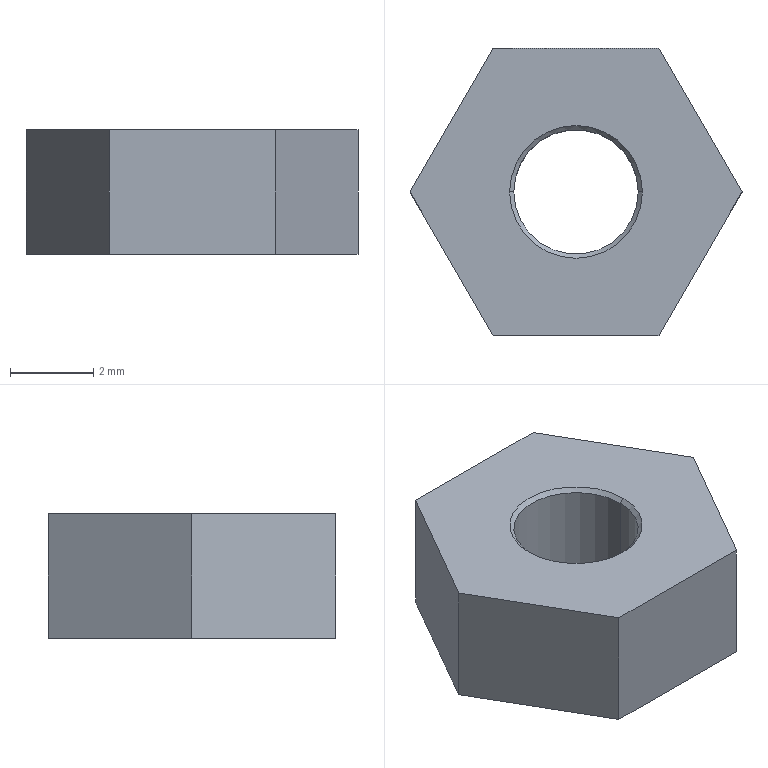Part | SolidWorks | features Chamfer 1, Extrusion 1 | 1 solid | 14 faces | box 8 x 6.928 x 3 mm | volume 103.406 mm3 | plane 8 | cone 4 | cylinder 2 | commonest cylinder face diameters 3 x2
STEP:
#1=CARTESIAN_POINT('',(-1.5,0.,2.9));
#2=VERTEX_POINT('',#1);
#3=CARTESIAN_POINT('',(1.5,0.,2.9));
#4=VERTEX_POINT('',#3);
#5=CARTESIAN_POINT('',(0.,0.,2.9));
#6=DIRECTION('',(0.,0.,1.));
#7=DIRECTION('',(1.,0.,0.));
#8=AXIS2_PLACEMENT_3D('',#5,#6,#7);
#9=CIRCLE('',#8,1.5);
#10=EDGE_CURVE('',#2,#4,#9,.T.);
#11=ORIENTED_EDGE('',*,*,#10,.F.);
#12=CARTESIAN_POINT('',(-1.6,0.,3.));
#13=VERTEX_POINT('',#12);
#14=CARTESIAN_POINT('',(-1.5,0.,2.9));
#15=DIRECTION('',(-0.7071,0.,0.7071));
#16=VECTOR('',#15,1000.);
#17=LINE('',#14,#16);
#18=EDGE_CURVE('',#2,#13,#17,.T.);
#19=ORIENTED_EDGE('',*,*,#18,.T.);
#20=CARTESIAN_POINT('',(1.6,0.,3.));
#21=VERTEX_POINT('',#20);
#22=CARTESIAN_POINT('',(0.,0.,3.));
#23=DIRECTION('',(0.,0.,-1.));
#24=DIRECTION('',(1.,0.,0.));
#25=AXIS2_PLACEMENT_3D('',#22,#23,#24);
#26=CIRCLE('',#25,1.6);
#27=EDGE_CURVE('',#21,#13,#26,.T.);
#28=ORIENTED_EDGE('',*,*,#27,.F.);
#29=CARTESIAN_POINT('',(1.5,0.,2.9));
#30=DIRECTION('',(0.7071,0.,0.7071));
#31=VECTOR('',#30,1000.);
#32=LINE('',#29,#31);
#33=EDGE_CURVE('',#4,#21,#32,.T.);
#34=ORIENTED_EDGE('',*,*,#33,.F.);
#35=EDGE_LOOP('',(#11,#19,#28,#34));
#36=FACE_OUTER_BOUND('',#35,.T.);
#37=CARTESIAN_POINT('',(0.,0.,2.9));
#38=DIRECTION('',(0.,0.,1.));
#39=DIRECTION('',(1.,0.,0.));
#40=AXIS2_PLACEMENT_3D('',#37,#38,#39);
#41=CONICAL_SURFACE('',#40,1.5,0.7854);
#42=ADVANCED_FACE('',(#36),#41,.F.);
#43=CARTESIAN_POINT('',(1.5,0.,0.1));
#44=VERTEX_POINT('',#43);
#45=CARTESIAN_POINT('',(-1.5,0.,0.1));
#46=VERTEX_POINT('',#45);
#47=CARTESIAN_POINT('',(0.,0.,0.1));
#48=DIRECTION('',(0.,0.,-1.));
#49=DIRECTION('',(1.,0.,0.));
#50=AXIS2_PLACEMENT_3D('',#47,#48,#49);
#51=CIRCLE('',#50,1.5);
#52=EDGE_CURVE('',#44,#46,#51,.T.);
#53=ORIENTED_EDGE('',*,*,#52,.F.);
#54=CARTESIAN_POINT('',(1.6,0.,0.));
#55=VERTEX_POINT('',#54);
#56=CARTESIAN_POINT('',(1.6,0.,0.));
#57=DIRECTION('',(0.7071,0.,-0.7071));
#58=VECTOR('',#57,1000.);
#59=LINE('',#56,#58);
#60=EDGE_CURVE('',#44,#55,#59,.T.);
#61=ORIENTED_EDGE('',*,*,#60,.T.);
#62=CARTESIAN_POINT('',(-1.6,0.,0.));
#63=VERTEX_POINT('',#62);
#64=CARTESIAN_POINT('',(0.,0.,0.));
#65=DIRECTION('',(0.,0.,1.));
#66=DIRECTION('',(1.,0.,0.));
#67=AXIS2_PLACEMENT_3D('',#64,#65,#66);
#68=CIRCLE('',#67,1.6);
#69=EDGE_CURVE('',#63,#55,#68,.T.);
#70=ORIENTED_EDGE('',*,*,#69,.F.);
#71=CARTESIAN_POINT('',(-1.6,0.,0.));
#72=DIRECTION('',(-0.7071,0.,-0.7071));
#73=VECTOR('',#72,1000.);
#74=LINE('',#71,#73);
#75=EDGE_CURVE('',#46,#63,#74,.T.);
#76=ORIENTED_EDGE('',*,*,#75,.F.);
#77=EDGE_LOOP('',(#53,#61,#70,#76));
#78=FACE_OUTER_BOUND('',#77,.T.);
#79=CARTESIAN_POINT('',(0.,0.,0.));
#80=DIRECTION('',(0.,0.,-1.));
#81=DIRECTION('',(-1.,0.,0.));
#82=AXIS2_PLACEMENT_3D('',#79,#80,#81);
#83=CONICAL_SURFACE('',#82,1.6,0.7854);
#84=ADVANCED_FACE('',(#78),#83,.F.);
#85=ORIENTED_EDGE('',*,*,#10,.T.);
#86=CARTESIAN_POINT('',(1.5,0.,3.));
#87=DIRECTION('',(0.,0.,-1.));
#88=VECTOR('',#87,1000.);
#89=LINE('',#86,#88);
#90=EDGE_CURVE('',#4,#44,#89,.T.);
#91=ORIENTED_EDGE('',*,*,#90,.T.);
#92=ORIENTED_EDGE('',*,*,#52,.T.);
#93=CARTESIAN_POINT('',(-1.5,0.,3.));
#94=DIRECTION('',(0.,0.,-1.));
#95=VECTOR('',#94,1000.);
#96=LINE('',#93,#95);
#97=EDGE_CURVE('',#2,#46,#96,.T.);
#98=ORIENTED_EDGE('',*,*,#97,.F.);
#99=EDGE_LOOP('',(#85,#91,#92,#98));
#100=FACE_OUTER_BOUND('',#99,.T.);
#101=CARTESIAN_POINT('',(0.,0.,3.));
#102=DIRECTION('',(0.,0.,-1.));
#103=DIRECTION('',(-1.,0.,0.));
#104=AXIS2_PLACEMENT_3D('',#101,#102,#103);
#105=CYLINDRICAL_SURFACE('',#104,1.5);
#106=ADVANCED_FACE('',(#100),#105,.F.);
#107=ORIENTED_EDGE('',*,*,#27,.T.);
#108=CARTESIAN_POINT('',(0.,0.,3.));
#109=DIRECTION('',(0.,0.,-1.));
#110=DIRECTION('',(1.,0.,0.));
#111=AXIS2_PLACEMENT_3D('',#108,#109,#110);
#112=CIRCLE('',#111,1.6);
#113=EDGE_CURVE('',#13,#21,#112,.T.);
#114=ORIENTED_EDGE('',*,*,#113,.T.);
#115=EDGE_LOOP('',(#107,#114));
#116=FACE_BOUND('',#115,.T.);
#117=CARTESIAN_POINT('',(-2.,-3.464,3.));
#118=VERTEX_POINT('',#117);
#119=CARTESIAN_POINT('',(2.,-3.464,3.));
#120=VERTEX_POINT('',#119);
#121=CARTESIAN_POINT('',(-2.,-3.464,3.));
#122=DIRECTION('',(1.,0.,0.));
#123=VECTOR('',#122,1000.);
#124=LINE('',#121,#123);
#125=EDGE_CURVE('',#118,#120,#124,.T.);
#126=ORIENTED_EDGE('',*,*,#125,.T.);
#127=CARTESIAN_POINT('',(4.,0.,3.));
#128=VERTEX_POINT('',#127);
#129=CARTESIAN_POINT('',(2.,-3.464,3.));
#130=DIRECTION('',(0.5,0.866,0.));
#131=VECTOR('',#130,1000.);
#132=LINE('',#129,#131);
#133=EDGE_CURVE('',#120,#128,#132,.T.);
#134=ORIENTED_EDGE('',*,*,#133,.T.);
#135=CARTESIAN_POINT('',(2.,3.464,3.));
#136=VERTEX_POINT('',#135);
#137=CARTESIAN_POINT('',(4.,0.,3.));
#138=DIRECTION('',(-0.5,0.866,0.));
#139=VECTOR('',#138,1000.);
#140=LINE('',#137,#139);
#141=EDGE_CURVE('',#128,#136,#140,.T.);
#142=ORIENTED_EDGE('',*,*,#141,.T.);
#143=CARTESIAN_POINT('',(-2.,3.464,3.));
#144=VERTEX_POINT('',#143);
#145=CARTESIAN_POINT('',(2.,3.464,3.));
#146=DIRECTION('',(-1.,0.,0.));
#147=VECTOR('',#146,1000.);
#148=LINE('',#145,#147);
#149=EDGE_CURVE('',#136,#144,#148,.T.);
#150=ORIENTED_EDGE('',*,*,#149,.T.);
#151=CARTESIAN_POINT('',(-4.,0.,3.));
#152=VERTEX_POINT('',#151);
#153=CARTESIAN_POINT('',(-2.,3.464,3.));
#154=DIRECTION('',(-0.5,-0.866,0.));
#155=VECTOR('',#154,1000.);
#156=LINE('',#153,#155);
#157=EDGE_CURVE('',#144,#152,#156,.T.);
#158=ORIENTED_EDGE('',*,*,#157,.T.);
#159=CARTESIAN_POINT('',(-4.,0.,3.));
#160=DIRECTION('',(0.5,-0.866,0.));
#161=VECTOR('',#160,1000.);
#162=LINE('',#159,#161);
#163=EDGE_CURVE('',#152,#118,#162,.T.);
#164=ORIENTED_EDGE('',*,*,#163,.T.);
#165=EDGE_LOOP('',(#126,#134,#142,#150,#158,#164));
#166=FACE_OUTER_BOUND('',#165,.T.);
#167=CARTESIAN_POINT('',(0.,0.,3.));
#168=DIRECTION('',(0.,0.,1.));
#169=DIRECTION('',(1.,0.,0.));
#170=AXIS2_PLACEMENT_3D('',#167,#168,#169);
#171=PLANE('',#170);
#172=ADVANCED_FACE('',(#116,#166),#171,.T.);
#173=ORIENTED_EDGE('',*,*,#69,.T.);
#174=CARTESIAN_POINT('',(0.,0.,0.));
#175=DIRECTION('',(0.,0.,1.));
#176=DIRECTION('',(1.,0.,0.));
#177=AXIS2_PLACEMENT_3D('',#174,#175,#176);
#178=CIRCLE('',#177,1.6);
#179=EDGE_CURVE('',#55,#63,#178,.T.);
#180=ORIENTED_EDGE('',*,*,#179,.T.);
#181=EDGE_LOOP('',(#173,#180));
#182=FACE_BOUND('',#181,.T.);
#183=CARTESIAN_POINT('',(-2.,-3.464,0.));
#184=VERTEX_POINT('',#183);
#185=CARTESIAN_POINT('',(2.,-3.464,0.));
#186=VERTEX_POINT('',#185);
#187=CARTESIAN_POINT('',(-2.,-3.464,0.));
#188=DIRECTION('',(1.,0.,0.));
#189=VECTOR('',#188,1000.);
#190=LINE('',#187,#189);
#191=EDGE_CURVE('',#184,#186,#190,.T.);
#192=ORIENTED_EDGE('',*,*,#191,.F.);
#193=CARTESIAN_POINT('',(-4.,0.,0.));
#194=VERTEX_POINT('',#193);
#195=CARTESIAN_POINT('',(-4.,0.,0.));
#196=DIRECTION('',(0.5,-0.866,0.));
#197=VECTOR('',#196,1000.);
#198=LINE('',#195,#197);
#199=EDGE_CURVE('',#194,#184,#198,.T.);
#200=ORIENTED_EDGE('',*,*,#199,.F.);
#201=CARTESIAN_POINT('',(-2.,3.464,0.));
#202=VERTEX_POINT('',#201);
#203=CARTESIAN_POINT('',(-2.,3.464,0.));
#204=DIRECTION('',(-0.5,-0.866,0.));
#205=VECTOR('',#204,1000.);
#206=LINE('',#203,#205);
#207=EDGE_CURVE('',#202,#194,#206,.T.);
#208=ORIENTED_EDGE('',*,*,#207,.F.);
#209=CARTESIAN_POINT('',(2.,3.464,0.));
#210=VERTEX_POINT('',#209);
#211=CARTESIAN_POINT('',(2.,3.464,0.));
#212=DIRECTION('',(-1.,0.,0.));
#213=VECTOR('',#212,1000.);
#214=LINE('',#211,#213);
#215=EDGE_CURVE('',#210,#202,#214,.T.);
#216=ORIENTED_EDGE('',*,*,#215,.F.);
#217=CARTESIAN_POINT('',(4.,0.,0.));
#218=VERTEX_POINT('',#217);
#219=CARTESIAN_POINT('',(4.,0.,0.));
#220=DIRECTION('',(-0.5,0.866,0.));
#221=VECTOR('',#220,1000.);
#222=LINE('',#219,#221);
#223=EDGE_CURVE('',#218,#210,#222,.T.);
#224=ORIENTED_EDGE('',*,*,#223,.F.);
#225=CARTESIAN_POINT('',(2.,-3.464,0.));
#226=DIRECTION('',(0.5,0.866,0.));
#227=VECTOR('',#226,1000.);
#228=LINE('',#225,#227);
#229=EDGE_CURVE('',#186,#218,#228,.T.);
#230=ORIENTED_EDGE('',*,*,#229,.F.);
#231=EDGE_LOOP('',(#192,#200,#208,#216,#224,#230));
#232=FACE_OUTER_BOUND('',#231,.T.);
#233=CARTESIAN_POINT('',(0.,0.,0.));
#234=DIRECTION('',(0.,0.,1.));
#235=DIRECTION('',(1.,0.,0.));
#236=AXIS2_PLACEMENT_3D('',#233,#234,#235);
#237=PLANE('',#236);
#238=ADVANCED_FACE('',(#182,#232),#237,.F.);
#239=ORIENTED_EDGE('',*,*,#191,.T.);
#240=CARTESIAN_POINT('',(2.,-3.464,3.));
#241=DIRECTION('',(0.,0.,-1.));
#242=VECTOR('',#241,1000.);
#243=LINE('',#240,#242);
#244=EDGE_CURVE('',#120,#186,#243,.T.);
#245=ORIENTED_EDGE('',*,*,#244,.F.);
#246=ORIENTED_EDGE('',*,*,#125,.F.);
#247=CARTESIAN_POINT('',(-2.,-3.464,3.));
#248=DIRECTION('',(0.,0.,-1.));
#249=VECTOR('',#248,1000.);
#250=LINE('',#247,#249);
#251=EDGE_CURVE('',#118,#184,#250,.T.);
#252=ORIENTED_EDGE('',*,*,#251,.T.);
#253=EDGE_LOOP('',(#239,#245,#246,#252));
#254=FACE_OUTER_BOUND('',#253,.T.);
#255=CARTESIAN_POINT('',(-2.,-3.464,3.));
#256=DIRECTION('',(0.,1.,0.));
#257=DIRECTION('',(-1.,0.,0.));
#258=AXIS2_PLACEMENT_3D('',#255,#256,#257);
#259=PLANE('',#258);
#260=ADVANCED_FACE('',(#254),#259,.F.);
#261=ORIENTED_EDGE('',*,*,#229,.T.);
#262=CARTESIAN_POINT('',(4.,0.,3.));
#263=DIRECTION('',(0.,0.,-1.));
#264=VECTOR('',#263,1000.);
#265=LINE('',#262,#264);
#266=EDGE_CURVE('',#128,#218,#265,.T.);
#267=ORIENTED_EDGE('',*,*,#266,.F.);
#268=ORIENTED_EDGE('',*,*,#133,.F.);
#269=ORIENTED_EDGE('',*,*,#244,.T.);
#270=EDGE_LOOP('',(#261,#267,#268,#269));
#271=FACE_OUTER_BOUND('',#270,.T.);
#272=CARTESIAN_POINT('',(2.,-3.464,3.));
#273=DIRECTION('',(-0.866,0.5,0.));
#274=DIRECTION('',(-0.5,-0.866,0.));
#275=AXIS2_PLACEMENT_3D('',#272,#273,#274);
#276=PLANE('',#275);
#277=ADVANCED_FACE('',(#271),#276,.F.);
#278=ORIENTED_EDGE('',*,*,#223,.T.);
#279=CARTESIAN_POINT('',(2.,3.464,3.));
#280=DIRECTION('',(0.,0.,-1.));
#281=VECTOR('',#280,1000.);
#282=LINE('',#279,#281);
#283=EDGE_CURVE('',#136,#210,#282,.T.);
#284=ORIENTED_EDGE('',*,*,#283,.F.);
#285=ORIENTED_EDGE('',*,*,#141,.F.);
#286=ORIENTED_EDGE('',*,*,#266,.T.);
#287=EDGE_LOOP('',(#278,#284,#285,#286));
#288=FACE_OUTER_BOUND('',#287,.T.);
#289=CARTESIAN_POINT('',(4.,0.,3.));
#290=DIRECTION('',(-0.866,-0.5,0.));
#291=DIRECTION('',(0.5,-0.866,0.));
#292=AXIS2_PLACEMENT_3D('',#289,#290,#291);
#293=PLANE('',#292);
#294=ADVANCED_FACE('',(#288),#293,.F.);
#295=ORIENTED_EDGE('',*,*,#215,.T.);
#296=CARTESIAN_POINT('',(-2.,3.464,3.));
#297=DIRECTION('',(0.,0.,-1.));
#298=VECTOR('',#297,1000.);
#299=LINE('',#296,#298);
#300=EDGE_CURVE('',#144,#202,#299,.T.);
#301=ORIENTED_EDGE('',*,*,#300,.F.);
#302=ORIENTED_EDGE('',*,*,#149,.F.);
#303=ORIENTED_EDGE('',*,*,#283,.T.);
#304=EDGE_LOOP('',(#295,#301,#302,#303));
#305=FACE_OUTER_BOUND('',#304,.T.);
#306=CARTESIAN_POINT('',(2.,3.464,3.));
#307=DIRECTION('',(0.,-1.,0.));
#308=DIRECTION('',(1.,0.,0.));
#309=AXIS2_PLACEMENT_3D('',#306,#307,#308);
#310=PLANE('',#309);
#311=ADVANCED_FACE('',(#305),#310,.F.);
#312=ORIENTED_EDGE('',*,*,#207,.T.);
#313=CARTESIAN_POINT('',(-4.,0.,3.));
#314=DIRECTION('',(0.,0.,-1.));
#315=VECTOR('',#314,1000.);
#316=LINE('',#313,#315);
#317=EDGE_CURVE('',#152,#194,#316,.T.);
#318=ORIENTED_EDGE('',*,*,#317,.F.);
#319=ORIENTED_EDGE('',*,*,#157,.F.);
#320=ORIENTED_EDGE('',*,*,#300,.T.);
#321=EDGE_LOOP('',(#312,#318,#319,#320));
#322=FACE_OUTER_BOUND('',#321,.T.);
#323=CARTESIAN_POINT('',(-2.,3.464,3.));
#324=DIRECTION('',(0.866,-0.5,0.));
#325=DIRECTION('',(0.5,0.866,0.));
#326=AXIS2_PLACEMENT_3D('',#323,#324,#325);
#327=PLANE('',#326);
#328=ADVANCED_FACE('',(#322),#327,.F.);
#329=ORIENTED_EDGE('',*,*,#199,.T.);
#330=ORIENTED_EDGE('',*,*,#251,.F.);
#331=ORIENTED_EDGE('',*,*,#163,.F.);
#332=ORIENTED_EDGE('',*,*,#317,.T.);
#333=EDGE_LOOP('',(#329,#330,#331,#332));
#334=FACE_OUTER_BOUND('',#333,.T.);
#335=CARTESIAN_POINT('',(-4.,0.,3.));
#336=DIRECTION('',(0.866,0.5,0.));
#337=DIRECTION('',(-0.5,0.866,0.));
#338=AXIS2_PLACEMENT_3D('',#335,#336,#337);
#339=PLANE('',#338);
#340=ADVANCED_FACE('',(#334),#339,.F.);
#341=ORIENTED_EDGE('',*,*,#90,.F.);
#342=CARTESIAN_POINT('',(0.,0.,2.9));
#343=DIRECTION('',(0.,0.,1.));
#344=DIRECTION('',(1.,0.,0.));
#345=AXIS2_PLACEMENT_3D('',#342,#343,#344);
#346=CIRCLE('',#345,1.5);
#347=EDGE_CURVE('',#4,#2,#346,.T.);
#348=ORIENTED_EDGE('',*,*,#347,.T.);
#349=ORIENTED_EDGE('',*,*,#97,.T.);
#350=CARTESIAN_POINT('',(0.,0.,0.1));
#351=DIRECTION('',(0.,0.,-1.));
#352=DIRECTION('',(1.,0.,0.));
#353=AXIS2_PLACEMENT_3D('',#350,#351,#352);
#354=CIRCLE('',#353,1.5);
#355=EDGE_CURVE('',#46,#44,#354,.T.);
#356=ORIENTED_EDGE('',*,*,#355,.T.);
#357=EDGE_LOOP('',(#341,#348,#349,#356));
#358=FACE_OUTER_BOUND('',#357,.T.);
#359=CARTESIAN_POINT('',(0.,0.,3.));
#360=DIRECTION('',(0.,0.,-1.));
#361=DIRECTION('',(-1.,0.,0.));
#362=AXIS2_PLACEMENT_3D('',#359,#360,#361);
#363=CYLINDRICAL_SURFACE('',#362,1.5);
#364=ADVANCED_FACE('',(#358),#363,.F.);
#365=ORIENTED_EDGE('',*,*,#60,.F.);
#366=ORIENTED_EDGE('',*,*,#355,.F.);
#367=ORIENTED_EDGE('',*,*,#75,.T.);
#368=ORIENTED_EDGE('',*,*,#179,.F.);
#369=EDGE_LOOP('',(#365,#366,#367,#368));
#370=FACE_OUTER_BOUND('',#369,.T.);
#371=CARTESIAN_POINT('',(0.,0.,0.));
#372=DIRECTION('',(0.,0.,-1.));
#373=DIRECTION('',(-1.,0.,0.));
#374=AXIS2_PLACEMENT_3D('',#371,#372,#373);
#375=CONICAL_SURFACE('',#374,1.6,0.7854);
#376=ADVANCED_FACE('',(#370),#375,.F.);
#377=ORIENTED_EDGE('',*,*,#18,.F.);
#378=ORIENTED_EDGE('',*,*,#347,.F.);
#379=ORIENTED_EDGE('',*,*,#33,.T.);
#380=ORIENTED_EDGE('',*,*,#113,.F.);
#381=EDGE_LOOP('',(#377,#378,#379,#380));
#382=FACE_OUTER_BOUND('',#381,.T.);
#383=CARTESIAN_POINT('',(0.,0.,2.9));
#384=DIRECTION('',(0.,0.,1.));
#385=DIRECTION('',(1.,0.,0.));
#386=AXIS2_PLACEMENT_3D('',#383,#384,#385);
#387=CONICAL_SURFACE('',#386,1.5,0.7854);
#388=ADVANCED_FACE('',(#382),#387,.F.);
#389=CLOSED_SHELL('',(#42,#84,#106,#172,#238,#260,#277,#294,#311,#328,#340,#364,#376,#388));
#390=MANIFOLD_SOLID_BREP('',#389);
#391=CARTESIAN_POINT('',(0.,0.,0.));
#392=DIRECTION('',(0.,0.,1.));
#393=DIRECTION('',(1.,0.,0.));
#394=AXIS2_PLACEMENT_3D('',#391,#392,#393);
#395=(LENGTH_UNIT()NAMED_UNIT(*)SI_UNIT(.MILLI.,.METRE.));
#396=UNCERTAINTY_MEASURE_WITH_UNIT(LENGTH_MEASURE(0.00001),#395,'','');
#397=(NAMED_UNIT(*)PLANE_ANGLE_UNIT()SI_UNIT($,.RADIAN.));
#398=(NAMED_UNIT(*)SI_UNIT($,.STERADIAN.)SOLID_ANGLE_UNIT());
#399=(GEOMETRIC_REPRESENTATION_CONTEXT(3)GLOBAL_UNCERTAINTY_ASSIGNED_CONTEXT((#396))GLOBAL_UNIT_ASSIGNED_CONTEXT((#395,#397,#398))REPRESENTATION_CONTEXT('',''));
#400=ADVANCED_BREP_SHAPE_REPRESENTATION('',(#390,#394),#399);